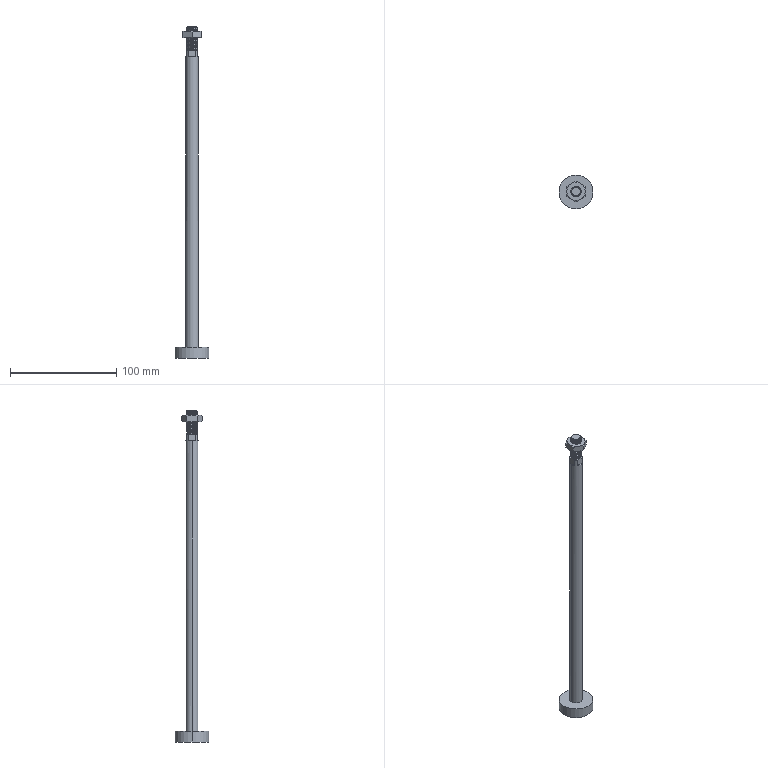Part | SolidWorks | features ICE 5, Revolution 3, RevCut 2, Chamfer 1, Helix 1, LPattern 1, MirrorPattern 1, SweepCut 1 | 1 solid | 74 faces | box 32 x 32 x 312.5 mm | volume 42170 mm3 | cylinder 32 | plane 23 | cone 15 | spline 4 | commonest cylinder face diameters 10 x26 8 x2 12 x2 32 x2